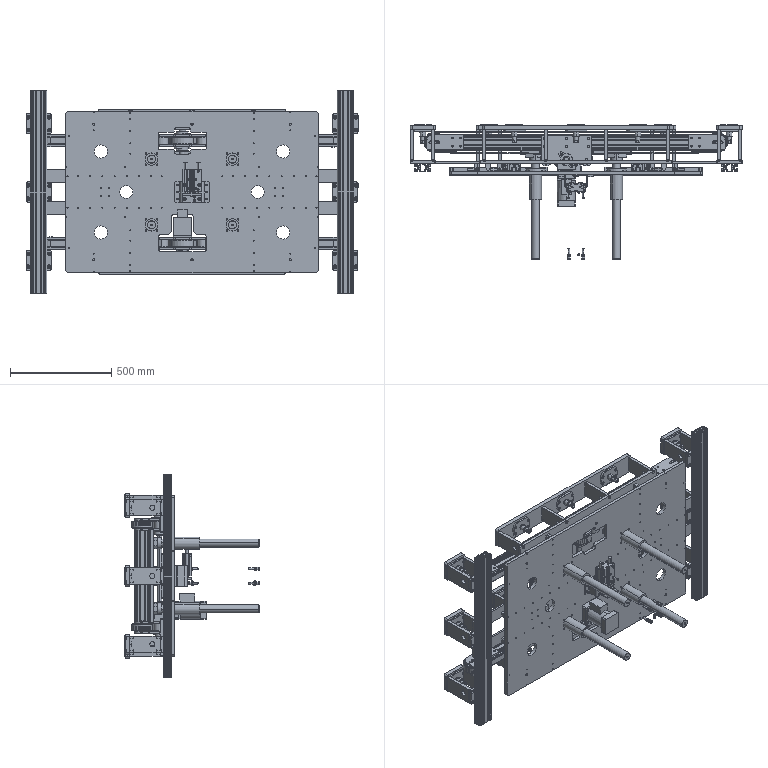Part | SolidWorks | features ReferencePattern 18, MirrorCompFeat 9 | 286 solids | 13783 faces | volume 55171435 mm3 | cylinder 5533 | plane 5416 | cone 1214 | torus 926 | sphere 512 | spline 182 | commonest cylinder face diameters 1.2 x452 1.6 x452 5 x406 9 x318 6.8 x316 6.6 x288